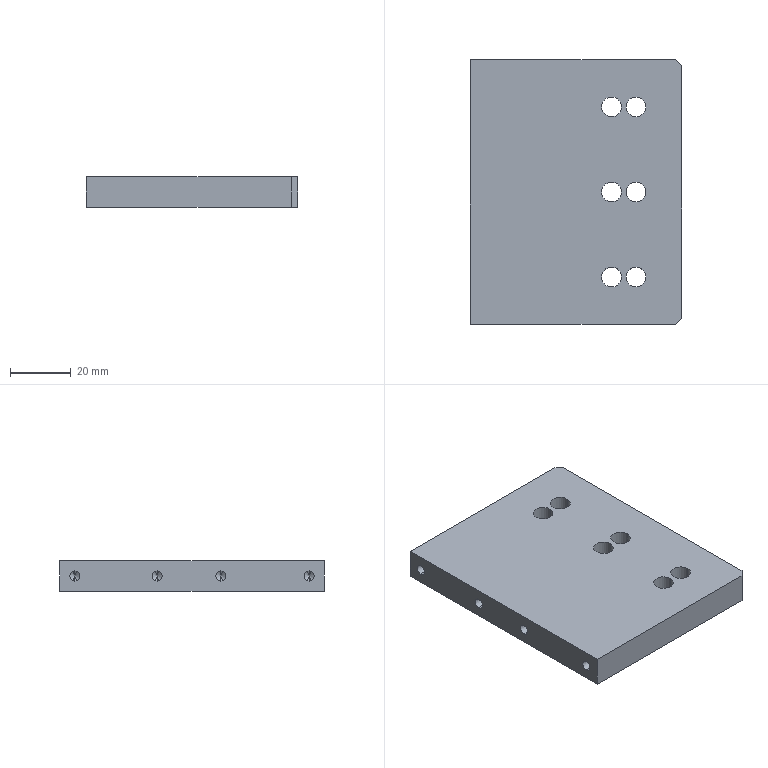Part | STEP file | 02-09 moving fixing plate | 1 solid | 36 faces | box 69.4 x 87 x 10 mm | volume 57942 mm3 | cylinder 20 | cone 8 | plane 8 | commonest cylinder face diameters 6.5 x12 3.3 x8
STEP:
#1=CARTESIAN_POINT('',(14.95,-28.,10.));
#2=VERTEX_POINT('',#1);
#3=CARTESIAN_POINT('',(8.45,-28.,10.));
#4=VERTEX_POINT('',#3);
#5=CARTESIAN_POINT('',(11.7,-28.,10.));
#6=DIRECTION('',(0.,0.,-1.));
#7=DIRECTION('',(-1.,0.,0.));
#8=AXIS2_PLACEMENT_3D('',#5,#6,#7);
#9=CIRCLE('',#8,3.25);
#10=EDGE_CURVE('',#2,#4,#9,.T.);
#11=ORIENTED_EDGE('',*,*,#10,.F.);
#12=CARTESIAN_POINT('',(14.95,-28.,0.));
#13=VERTEX_POINT('',#12);
#14=CARTESIAN_POINT('',(14.95,-28.,10.));
#15=DIRECTION('',(0.,0.,-1.));
#16=VECTOR('',#15,1000.);
#17=LINE('',#14,#16);
#18=EDGE_CURVE('',#2,#13,#17,.T.);
#19=ORIENTED_EDGE('',*,*,#18,.T.);
#20=CARTESIAN_POINT('',(8.45,-28.,0.));
#21=VERTEX_POINT('',#20);
#22=CARTESIAN_POINT('',(11.7,-28.,0.));
#23=DIRECTION('',(0.,0.,-1.));
#24=DIRECTION('',(-1.,0.,0.));
#25=AXIS2_PLACEMENT_3D('',#22,#23,#24);
#26=CIRCLE('',#25,3.25);
#27=EDGE_CURVE('',#13,#21,#26,.T.);
#28=ORIENTED_EDGE('',*,*,#27,.T.);
#29=CARTESIAN_POINT('',(8.45,-28.,10.));
#30=DIRECTION('',(0.,0.,-1.));
#31=VECTOR('',#30,1000.);
#32=LINE('',#29,#31);
#33=EDGE_CURVE('',#4,#21,#32,.T.);
#34=ORIENTED_EDGE('',*,*,#33,.F.);
#35=EDGE_LOOP('',(#11,#19,#28,#34));
#36=FACE_OUTER_BOUND('',#35,.T.);
#37=CARTESIAN_POINT('',(11.7,-28.,10.));
#38=DIRECTION('',(0.,0.,-1.));
#39=DIRECTION('',(-1.,0.,0.));
#40=AXIS2_PLACEMENT_3D('',#37,#38,#39);
#41=CYLINDRICAL_SURFACE('',#40,3.25);
#42=ADVANCED_FACE('',(#36),#41,.F.);
#43=CARTESIAN_POINT('',(14.95,0.,10.));
#44=VERTEX_POINT('',#43);
#45=CARTESIAN_POINT('',(8.45,0.,10.));
#46=VERTEX_POINT('',#45);
#47=CARTESIAN_POINT('',(11.7,0.,10.));
#48=DIRECTION('',(0.,0.,-1.));
#49=DIRECTION('',(-1.,0.,0.));
#50=AXIS2_PLACEMENT_3D('',#47,#48,#49);
#51=CIRCLE('',#50,3.25);
#52=EDGE_CURVE('',#44,#46,#51,.T.);
#53=ORIENTED_EDGE('',*,*,#52,.F.);
#54=CARTESIAN_POINT('',(14.95,0.,0.));
#55=VERTEX_POINT('',#54);
#56=CARTESIAN_POINT('',(14.95,0.,10.));
#57=DIRECTION('',(0.,0.,-1.));
#58=VECTOR('',#57,1000.);
#59=LINE('',#56,#58);
#60=EDGE_CURVE('',#44,#55,#59,.T.);
#61=ORIENTED_EDGE('',*,*,#60,.T.);
#62=CARTESIAN_POINT('',(8.45,0.,0.));
#63=VERTEX_POINT('',#62);
#64=CARTESIAN_POINT('',(11.7,0.,0.));
#65=DIRECTION('',(0.,0.,-1.));
#66=DIRECTION('',(-1.,0.,0.));
#67=AXIS2_PLACEMENT_3D('',#64,#65,#66);
#68=CIRCLE('',#67,3.25);
#69=EDGE_CURVE('',#55,#63,#68,.T.);
#70=ORIENTED_EDGE('',*,*,#69,.T.);
#71=CARTESIAN_POINT('',(8.45,0.,10.));
#72=DIRECTION('',(0.,0.,-1.));
#73=VECTOR('',#72,1000.);
#74=LINE('',#71,#73);
#75=EDGE_CURVE('',#46,#63,#74,.T.);
#76=ORIENTED_EDGE('',*,*,#75,.F.);
#77=EDGE_LOOP('',(#53,#61,#70,#76));
#78=FACE_OUTER_BOUND('',#77,.T.);
#79=CARTESIAN_POINT('',(11.7,0.,10.));
#80=DIRECTION('',(0.,0.,-1.));
#81=DIRECTION('',(-1.,0.,0.));
#82=AXIS2_PLACEMENT_3D('',#79,#80,#81);
#83=CYLINDRICAL_SURFACE('',#82,3.25);
#84=ADVANCED_FACE('',(#78),#83,.F.);
#85=CARTESIAN_POINT('',(14.95,28.,10.));
#86=VERTEX_POINT('',#85);
#87=CARTESIAN_POINT('',(8.45,28.,10.));
#88=VERTEX_POINT('',#87);
#89=CARTESIAN_POINT('',(11.7,28.,10.));
#90=DIRECTION('',(0.,0.,-1.));
#91=DIRECTION('',(-1.,0.,0.));
#92=AXIS2_PLACEMENT_3D('',#89,#90,#91);
#93=CIRCLE('',#92,3.25);
#94=EDGE_CURVE('',#86,#88,#93,.T.);
#95=ORIENTED_EDGE('',*,*,#94,.F.);
#96=CARTESIAN_POINT('',(14.95,28.,0.));
#97=VERTEX_POINT('',#96);
#98=CARTESIAN_POINT('',(14.95,28.,10.));
#99=DIRECTION('',(0.,0.,-1.));
#100=VECTOR('',#99,1000.);
#101=LINE('',#98,#100);
#102=EDGE_CURVE('',#86,#97,#101,.T.);
#103=ORIENTED_EDGE('',*,*,#102,.T.);
#104=CARTESIAN_POINT('',(8.45,28.,0.));
#105=VERTEX_POINT('',#104);
#106=CARTESIAN_POINT('',(11.7,28.,0.));
#107=DIRECTION('',(0.,0.,-1.));
#108=DIRECTION('',(-1.,0.,0.));
#109=AXIS2_PLACEMENT_3D('',#106,#107,#108);
#110=CIRCLE('',#109,3.25);
#111=EDGE_CURVE('',#97,#105,#110,.T.);
#112=ORIENTED_EDGE('',*,*,#111,.T.);
#113=CARTESIAN_POINT('',(8.45,28.,10.));
#114=DIRECTION('',(0.,0.,-1.));
#115=VECTOR('',#114,1000.);
#116=LINE('',#113,#115);
#117=EDGE_CURVE('',#88,#105,#116,.T.);
#118=ORIENTED_EDGE('',*,*,#117,.F.);
#119=EDGE_LOOP('',(#95,#103,#112,#118));
#120=FACE_OUTER_BOUND('',#119,.T.);
#121=CARTESIAN_POINT('',(11.7,28.,10.));
#122=DIRECTION('',(0.,0.,-1.));
#123=DIRECTION('',(-1.,0.,0.));
#124=AXIS2_PLACEMENT_3D('',#121,#122,#123);
#125=CYLINDRICAL_SURFACE('',#124,3.25);
#126=ADVANCED_FACE('',(#120),#125,.F.);
#127=CARTESIAN_POINT('',(16.45,-28.,0.));
#128=VERTEX_POINT('',#127);
#129=CARTESIAN_POINT('',(22.95,-28.,0.));
#130=VERTEX_POINT('',#129);
#131=CARTESIAN_POINT('',(19.7,-28.,0.));
#132=DIRECTION('',(0.,0.,1.));
#133=DIRECTION('',(1.,0.,0.));
#134=AXIS2_PLACEMENT_3D('',#131,#132,#133);
#135=CIRCLE('',#134,3.25);
#136=EDGE_CURVE('',#128,#130,#135,.T.);
#137=ORIENTED_EDGE('',*,*,#136,.F.);
#138=CARTESIAN_POINT('',(16.45,-28.,10.));
#139=VERTEX_POINT('',#138);
#140=CARTESIAN_POINT('',(16.45,-28.,0.));
#141=DIRECTION('',(0.,0.,1.));
#142=VECTOR('',#141,1000.);
#143=LINE('',#140,#142);
#144=EDGE_CURVE('',#128,#139,#143,.T.);
#145=ORIENTED_EDGE('',*,*,#144,.T.);
#146=CARTESIAN_POINT('',(22.95,-28.,10.));
#147=VERTEX_POINT('',#146);
#148=CARTESIAN_POINT('',(19.7,-28.,10.));
#149=DIRECTION('',(0.,0.,1.));
#150=DIRECTION('',(1.,0.,0.));
#151=AXIS2_PLACEMENT_3D('',#148,#149,#150);
#152=CIRCLE('',#151,3.25);
#153=EDGE_CURVE('',#139,#147,#152,.T.);
#154=ORIENTED_EDGE('',*,*,#153,.T.);
#155=CARTESIAN_POINT('',(22.95,-28.,0.));
#156=DIRECTION('',(0.,0.,1.));
#157=VECTOR('',#156,1000.);
#158=LINE('',#155,#157);
#159=EDGE_CURVE('',#130,#147,#158,.T.);
#160=ORIENTED_EDGE('',*,*,#159,.F.);
#161=EDGE_LOOP('',(#137,#145,#154,#160));
#162=FACE_OUTER_BOUND('',#161,.T.);
#163=CARTESIAN_POINT('',(19.7,-28.,0.));
#164=DIRECTION('',(0.,0.,1.));
#165=DIRECTION('',(1.,0.,0.));
#166=AXIS2_PLACEMENT_3D('',#163,#164,#165);
#167=CYLINDRICAL_SURFACE('',#166,3.25);
#168=ADVANCED_FACE('',(#162),#167,.F.);
#169=CARTESIAN_POINT('',(16.45,0.,0.));
#170=VERTEX_POINT('',#169);
#171=CARTESIAN_POINT('',(22.95,0.,0.));
#172=VERTEX_POINT('',#171);
#173=CARTESIAN_POINT('',(19.7,0.,0.));
#174=DIRECTION('',(0.,0.,1.));
#175=DIRECTION('',(1.,0.,0.));
#176=AXIS2_PLACEMENT_3D('',#173,#174,#175);
#177=CIRCLE('',#176,3.25);
#178=EDGE_CURVE('',#170,#172,#177,.T.);
#179=ORIENTED_EDGE('',*,*,#178,.F.);
#180=CARTESIAN_POINT('',(16.45,0.,10.));
#181=VERTEX_POINT('',#180);
#182=CARTESIAN_POINT('',(16.45,0.,0.));
#183=DIRECTION('',(0.,0.,1.));
#184=VECTOR('',#183,1000.);
#185=LINE('',#182,#184);
#186=EDGE_CURVE('',#170,#181,#185,.T.);
#187=ORIENTED_EDGE('',*,*,#186,.T.);
#188=CARTESIAN_POINT('',(22.95,0.,10.));
#189=VERTEX_POINT('',#188);
#190=CARTESIAN_POINT('',(19.7,0.,10.));
#191=DIRECTION('',(0.,0.,1.));
#192=DIRECTION('',(1.,0.,0.));
#193=AXIS2_PLACEMENT_3D('',#190,#191,#192);
#194=CIRCLE('',#193,3.25);
#195=EDGE_CURVE('',#181,#189,#194,.T.);
#196=ORIENTED_EDGE('',*,*,#195,.T.);
#197=CARTESIAN_POINT('',(22.95,0.,0.));
#198=DIRECTION('',(0.,0.,1.));
#199=VECTOR('',#198,1000.);
#200=LINE('',#197,#199);
#201=EDGE_CURVE('',#172,#189,#200,.T.);
#202=ORIENTED_EDGE('',*,*,#201,.F.);
#203=EDGE_LOOP('',(#179,#187,#196,#202));
#204=FACE_OUTER_BOUND('',#203,.T.);
#205=CARTESIAN_POINT('',(19.7,0.,0.));
#206=DIRECTION('',(0.,0.,1.));
#207=DIRECTION('',(1.,0.,0.));
#208=AXIS2_PLACEMENT_3D('',#205,#206,#207);
#209=CYLINDRICAL_SURFACE('',#208,3.25);
#210=ADVANCED_FACE('',(#204),#209,.F.);
#211=CARTESIAN_POINT('',(16.45,28.,0.));
#212=VERTEX_POINT('',#211);
#213=CARTESIAN_POINT('',(22.95,28.,0.));
#214=VERTEX_POINT('',#213);
#215=CARTESIAN_POINT('',(19.7,28.,0.));
#216=DIRECTION('',(0.,0.,1.));
#217=DIRECTION('',(1.,0.,0.));
#218=AXIS2_PLACEMENT_3D('',#215,#216,#217);
#219=CIRCLE('',#218,3.25);
#220=EDGE_CURVE('',#212,#214,#219,.T.);
#221=ORIENTED_EDGE('',*,*,#220,.F.);
#222=CARTESIAN_POINT('',(16.45,28.,10.));
#223=VERTEX_POINT('',#222);
#224=CARTESIAN_POINT('',(16.45,28.,0.));
#225=DIRECTION('',(0.,0.,1.));
#226=VECTOR('',#225,1000.);
#227=LINE('',#224,#226);
#228=EDGE_CURVE('',#212,#223,#227,.T.);
#229=ORIENTED_EDGE('',*,*,#228,.T.);
#230=CARTESIAN_POINT('',(22.95,28.,10.));
#231=VERTEX_POINT('',#230);
#232=CARTESIAN_POINT('',(19.7,28.,10.));
#233=DIRECTION('',(0.,0.,1.));
#234=DIRECTION('',(1.,0.,0.));
#235=AXIS2_PLACEMENT_3D('',#232,#233,#234);
#236=CIRCLE('',#235,3.25);
#237=EDGE_CURVE('',#223,#231,#236,.T.);
#238=ORIENTED_EDGE('',*,*,#237,.T.);
#239=CARTESIAN_POINT('',(22.95,28.,0.));
#240=DIRECTION('',(0.,0.,1.));
#241=VECTOR('',#240,1000.);
#242=LINE('',#239,#241);
#243=EDGE_CURVE('',#214,#231,#242,.T.);
#244=ORIENTED_EDGE('',*,*,#243,.F.);
#245=EDGE_LOOP('',(#221,#229,#238,#244));
#246=FACE_OUTER_BOUND('',#245,.T.);
#247=CARTESIAN_POINT('',(19.7,28.,0.));
#248=DIRECTION('',(0.,0.,1.));
#249=DIRECTION('',(1.,0.,0.));
#250=AXIS2_PLACEMENT_3D('',#247,#248,#249);
#251=CYLINDRICAL_SURFACE('',#250,3.25);
#252=ADVANCED_FACE('',(#246),#251,.F.);
#253=CARTESIAN_POINT('',(-23.2,38.5,3.35));
#254=VERTEX_POINT('',#253);
#255=CARTESIAN_POINT('',(-23.2,38.5,6.65));
#256=VERTEX_POINT('',#255);
#257=CARTESIAN_POINT('',(-23.2,38.5,5.));
#258=DIRECTION('',(-1.,0.,0.));
#259=DIRECTION('',(0.,0.,1.));
#260=AXIS2_PLACEMENT_3D('',#257,#258,#259);
#261=CIRCLE('',#260,1.65);
#262=EDGE_CURVE('',#254,#256,#261,.T.);
#263=ORIENTED_EDGE('',*,*,#262,.F.);
#264=CARTESIAN_POINT('',(-34.7,38.5,3.35));
#265=VERTEX_POINT('',#264);
#266=CARTESIAN_POINT('',(-34.7,38.5,3.35));
#267=DIRECTION('',(-1.,0.,0.));
#268=VECTOR('',#267,1000.);
#269=LINE('',#266,#268);
#270=EDGE_CURVE('',#254,#265,#269,.T.);
#271=ORIENTED_EDGE('',*,*,#270,.T.);
#272=CARTESIAN_POINT('',(-34.7,38.5,6.65));
#273=VERTEX_POINT('',#272);
#274=CARTESIAN_POINT('',(-34.7,38.5,5.));
#275=DIRECTION('',(-1.,0.,0.));
#276=DIRECTION('',(0.,0.,1.));
#277=AXIS2_PLACEMENT_3D('',#274,#275,#276);
#278=CIRCLE('',#277,1.65);
#279=EDGE_CURVE('',#265,#273,#278,.T.);
#280=ORIENTED_EDGE('',*,*,#279,.T.);
#281=CARTESIAN_POINT('',(-34.7,38.5,6.65));
#282=DIRECTION('',(-1.,0.,0.));
#283=VECTOR('',#282,1000.);
#284=LINE('',#281,#283);
#285=EDGE_CURVE('',#256,#273,#284,.T.);
#286=ORIENTED_EDGE('',*,*,#285,.F.);
#287=EDGE_LOOP('',(#263,#271,#280,#286));
#288=FACE_OUTER_BOUND('',#287,.T.);
#289=CARTESIAN_POINT('',(-34.7,38.5,5.));
#290=DIRECTION('',(-1.,0.,0.));
#291=DIRECTION('',(0.,0.,1.));
#292=AXIS2_PLACEMENT_3D('',#289,#290,#291);
#293=CYLINDRICAL_SURFACE('',#292,1.65);
#294=ADVANCED_FACE('',(#288),#293,.F.);
#295=CARTESIAN_POINT('',(-22.209,38.5,5.));
#296=VERTEX_POINT('',#295);
#297=CARTESIAN_POINT('',(-23.2,38.5,6.65));
#298=DIRECTION('',(-0.515,0.,0.8572));
#299=VECTOR('',#298,1000.);
#300=LINE('',#297,#299);
#301=EDGE_CURVE('',#296,#256,#300,.T.);
#302=ORIENTED_EDGE('',*,*,#301,.F.);
#303=CARTESIAN_POINT('',(-23.2,38.5,3.35));
#304=DIRECTION('',(-0.515,0.,-0.8572));
#305=VECTOR('',#304,1000.);
#306=LINE('',#303,#305);
#307=EDGE_CURVE('',#296,#254,#306,.T.);
#308=ORIENTED_EDGE('',*,*,#307,.T.);
#309=ORIENTED_EDGE('',*,*,#262,.T.);
#310=EDGE_LOOP('',(#302,#308,#309));
#311=FACE_OUTER_BOUND('',#310,.T.);
#312=CARTESIAN_POINT('',(-23.2,38.5,5.));
#313=DIRECTION('',(-1.,0.,0.));
#314=DIRECTION('',(0.,0.,1.));
#315=AXIS2_PLACEMENT_3D('',#312,#313,#314);
#316=CONICAL_SURFACE('',#315,1.65,1.03);
#317=ADVANCED_FACE('',(#311),#316,.F.);
#318=CARTESIAN_POINT('',(-23.2,-38.5,3.35));
#319=VERTEX_POINT('',#318);
#320=CARTESIAN_POINT('',(-23.2,-38.5,6.65));
#321=VERTEX_POINT('',#320);
#322=CARTESIAN_POINT('',(-23.2,-38.5,5.));
#323=DIRECTION('',(-1.,0.,0.));
#324=DIRECTION('',(0.,0.,1.));
#325=AXIS2_PLACEMENT_3D('',#322,#323,#324);
#326=CIRCLE('',#325,1.65);
#327=EDGE_CURVE('',#319,#321,#326,.T.);
#328=ORIENTED_EDGE('',*,*,#327,.F.);
#329=CARTESIAN_POINT('',(-34.7,-38.5,3.35));
#330=VERTEX_POINT('',#329);
#331=CARTESIAN_POINT('',(-34.7,-38.5,3.35));
#332=DIRECTION('',(-1.,0.,0.));
#333=VECTOR('',#332,1000.);
#334=LINE('',#331,#333);
#335=EDGE_CURVE('',#319,#330,#334,.T.);
#336=ORIENTED_EDGE('',*,*,#335,.T.);
#337=CARTESIAN_POINT('',(-34.7,-38.5,6.65));
#338=VERTEX_POINT('',#337);
#339=CARTESIAN_POINT('',(-34.7,-38.5,5.));
#340=DIRECTION('',(-1.,0.,0.));
#341=DIRECTION('',(0.,0.,1.));
#342=AXIS2_PLACEMENT_3D('',#339,#340,#341);
#343=CIRCLE('',#342,1.65);
#344=EDGE_CURVE('',#330,#338,#343,.T.);
#345=ORIENTED_EDGE('',*,*,#344,.T.);
#346=CARTESIAN_POINT('',(-34.7,-38.5,6.65));
#347=DIRECTION('',(-1.,0.,0.));
#348=VECTOR('',#347,1000.);
#349=LINE('',#346,#348);
#350=EDGE_CURVE('',#321,#338,#349,.T.);
#351=ORIENTED_EDGE('',*,*,#350,.F.);
#352=EDGE_LOOP('',(#328,#336,#345,#351));
#353=FACE_OUTER_BOUND('',#352,.T.);
#354=CARTESIAN_POINT('',(-34.7,-38.5,5.));
#355=DIRECTION('',(-1.,0.,0.));
#356=DIRECTION('',(0.,0.,1.));
#357=AXIS2_PLACEMENT_3D('',#354,#355,#356);
#358=CYLINDRICAL_SURFACE('',#357,1.65);
#359=ADVANCED_FACE('',(#353),#358,.F.);
#360=CARTESIAN_POINT('',(-22.209,-38.5,5.));
#361=VERTEX_POINT('',#360);
#362=CARTESIAN_POINT('',(-23.2,-38.5,6.65));
#363=DIRECTION('',(-0.515,0.,0.8572));
#364=VECTOR('',#363,1000.);
#365=LINE('',#362,#364);
#366=EDGE_CURVE('',#361,#321,#365,.T.);
#367=ORIENTED_EDGE('',*,*,#366,.F.);
#368=CARTESIAN_POINT('',(-23.2,-38.5,3.35));
#369=DIRECTION('',(-0.515,0.,-0.8572));
#370=VECTOR('',#369,1000.);
#371=LINE('',#368,#370);
#372=EDGE_CURVE('',#361,#319,#371,.T.);
#373=ORIENTED_EDGE('',*,*,#372,.T.);
#374=ORIENTED_EDGE('',*,*,#327,.T.);
#375=EDGE_LOOP('',(#367,#373,#374));
#376=FACE_OUTER_BOUND('',#375,.T.);
#377=CARTESIAN_POINT('',(-23.2,-38.5,5.));
#378=DIRECTION('',(-1.,0.,0.));
#379=DIRECTION('',(0.,0.,1.));
#380=AXIS2_PLACEMENT_3D('',#377,#378,#379);
#381=CONICAL_SURFACE('',#380,1.65,1.03);
#382=ADVANCED_FACE('',(#376),#381,.F.);
#383=CARTESIAN_POINT('',(-23.2,11.5,3.35));
#384=VERTEX_POINT('',#383);
#385=CARTESIAN_POINT('',(-23.2,11.5,6.65));
#386=VERTEX_POINT('',#385);
#387=CARTESIAN_POINT('',(-23.2,11.5,5.));
#388=DIRECTION('',(-1.,0.,0.));
#389=DIRECTION('',(0.,0.,1.));
#390=AXIS2_PLACEMENT_3D('',#387,#388,#389);
#391=CIRCLE('',#390,1.65);
#392=EDGE_CURVE('',#384,#386,#391,.T.);
#393=ORIENTED_EDGE('',*,*,#392,.F.);
#394=CARTESIAN_POINT('',(-34.7,11.5,3.35));
#395=VERTEX_POINT('',#394);
#396=CARTESIAN_POINT('',(-34.7,11.5,3.35));
#397=DIRECTION('',(-1.,0.,0.));
#398=VECTOR('',#397,1000.);
#399=LINE('',#396,#398);
#400=EDGE_CURVE('',#384,#395,#399,.T.);
#401=ORIENTED_EDGE('',*,*,#400,.T.);
#402=CARTESIAN_POINT('',(-34.7,11.5,6.65));
#403=VERTEX_POINT('',#402);
#404=CARTESIAN_POINT('',(-34.7,11.5,5.));
#405=DIRECTION('',(-1.,0.,0.));
#406=DIRECTION('',(0.,0.,1.));
#407=AXIS2_PLACEMENT_3D('',#404,#405,#406);
#408=CIRCLE('',#407,1.65);
#409=EDGE_CURVE('',#395,#403,#408,.T.);
#410=ORIENTED_EDGE('',*,*,#409,.T.);
#411=CARTESIAN_POINT('',(-34.7,11.5,6.65));
#412=DIRECTION('',(-1.,0.,0.));
#413=VECTOR('',#412,1000.);
#414=LINE('',#411,#413);
#415=EDGE_CURVE('',#386,#403,#414,.T.);
#416=ORIENTED_EDGE('',*,*,#415,.F.);
#417=EDGE_LOOP('',(#393,#401,#410,#416));
#418=FACE_OUTER_BOUND('',#417,.T.);
#419=CARTESIAN_POINT('',(-34.7,11.5,5.));
#420=DIRECTION('',(-1.,0.,0.));
#421=DIRECTION('',(0.,0.,1.));
#422=AXIS2_PLACEMENT_3D('',#419,#420,#421);
#423=CYLINDRICAL_SURFACE('',#422,1.65);
#424=ADVANCED_FACE('',(#418),#423,.F.);
#425=CARTESIAN_POINT('',(-22.209,11.5,5.));
#426=VERTEX_POINT('',#425);
#427=CARTESIAN_POINT('',(-23.2,11.5,6.65));
#428=DIRECTION('',(-0.515,0.,0.8572));
#429=VECTOR('',#428,1000.);
#430=LINE('',#427,#429);
#431=EDGE_CURVE('',#426,#386,#430,.T.);
#432=ORIENTED_EDGE('',*,*,#431,.F.);
#433=CARTESIAN_POINT('',(-23.2,11.5,3.35));
#434=DIRECTION('',(-0.515,0.,-0.8572));
#435=VECTOR('',#434,1000.);
#436=LINE('',#433,#435);
#437=EDGE_CURVE('',#426,#384,#436,.T.);
#438=ORIENTED_EDGE('',*,*,#437,.T.);
#439=ORIENTED_EDGE('',*,*,#392,.T.);
#440=EDGE_LOOP('',(#432,#438,#439));
#441=FACE_OUTER_BOUND('',#440,.T.);
#442=CARTESIAN_POINT('',(-23.2,11.5,5.));
#443=DIRECTION('',(-1.,0.,0.));
#444=DIRECTION('',(0.,0.,1.));
#445=AXIS2_PLACEMENT_3D('',#442,#443,#444);
#446=CONICAL_SURFACE('',#445,1.65,1.03);
#447=ADVANCED_FACE('',(#441),#446,.F.);
#448=CARTESIAN_POINT('',(-23.2,-9.5,3.35));
#449=VERTEX_POINT('',#448);
#450=CARTESIAN_POINT('',(-23.2,-9.5,6.65));
#451=VERTEX_POINT('',#450);
#452=CARTESIAN_POINT('',(-23.2,-9.5,5.));
#453=DIRECTION('',(-1.,0.,0.));
#454=DIRECTION('',(0.,0.,1.));
#455=AXIS2_PLACEMENT_3D('',#452,#453,#454);
#456=CIRCLE('',#455,1.65);
#457=EDGE_CURVE('',#449,#451,#456,.T.);
#458=ORIENTED_EDGE('',*,*,#457,.F.);
#459=CARTESIAN_POINT('',(-34.7,-9.5,3.35));
#460=VERTEX_POINT('',#459);
#461=CARTESIAN_POINT('',(-34.7,-9.5,3.35));
#462=DIRECTION('',(-1.,0.,0.));
#463=VECTOR('',#462,1000.);
#464=LINE('',#461,#463);
#465=EDGE_CURVE('',#449,#460,#464,.T.);
#466=ORIENTED_EDGE('',*,*,#465,.T.);
#467=CARTESIAN_POINT('',(-34.7,-9.5,6.65));
#468=VERTEX_POINT('',#467);
#469=CARTESIAN_POINT('',(-34.7,-9.5,5.));
#470=DIRECTION('',(-1.,0.,0.));
#471=DIRECTION('',(0.,0.,1.));
#472=AXIS2_PLACEMENT_3D('',#469,#470,#471);
#473=CIRCLE('',#472,1.65);
#474=EDGE_CURVE('',#460,#468,#473,.T.);
#475=ORIENTED_EDGE('',*,*,#474,.T.);
#476=CARTESIAN_POINT('',(-34.7,-9.5,6.65));
#477=DIRECTION('',(-1.,0.,0.));
#478=VECTOR('',#477,1000.);
#479=LINE('',#476,#478);
#480=EDGE_CURVE('',#451,#468,#479,.T.);
#481=ORIENTED_EDGE('',*,*,#480,.F.);
#482=EDGE_LOOP('',(#458,#466,#475,#481));
#483=FACE_OUTER_BOUND('',#482,.T.);
#484=CARTESIAN_POINT('',(-34.7,-9.5,5.));
#485=DIRECTION('',(-1.,0.,0.));
#486=DIRECTION('',(0.,0.,1.));
#487=AXIS2_PLACEMENT_3D('',#484,#485,#486);
#488=CYLINDRICAL_SURFACE('',#487,1.65);
#489=ADVANCED_FACE('',(#483),#488,.F.);
#490=CARTESIAN_POINT('',(-22.209,-9.5,5.));
#491=VERTEX_POINT('',#490);
#492=CARTESIAN_POINT('',(-23.2,-9.5,6.65));
#493=DIRECTION('',(-0.515,0.,0.8572));
#494=VECTOR('',#493,1000.);
#495=LINE('',#492,#494);
#496=EDGE_CURVE('',#491,#451,#495,.T.);
#497=ORIENTED_EDGE('',*,*,#496,.F.);
#498=CARTESIAN_POINT('',(-23.2,-9.5,3.35));
#499=DIRECTION('',(-0.515,0.,-0.8572));
#500=VECTOR('',#499,1000.);
#501=LINE('',#498,#500);
#502=EDGE_CURVE('',#491,#449,#501,.T.);
#503=ORIENTED_EDGE('',*,*,#502,.T.);
#504=ORIENTED_EDGE('',*,*,#457,.T.);
#505=EDGE_LOOP('',(#497,#503,#504));
#506=FACE_OUTER_BOUND('',#505,.T.);
#507=CARTESIAN_POINT('',(-23.2,-9.5,5.));
#508=DIRECTION('',(-1.,0.,0.));
#509=DIRECTION('',(0.,0.,1.));
#510=AXIS2_PLACEMENT_3D('',#507,#508,#509);
#511=CONICAL_SURFACE('',#510,1.65,1.03);
#512=ADVANCED_FACE('',(#506),#511,.F.);
#513=CARTESIAN_POINT('',(34.7,-41.5,0.));
#514=VERTEX_POINT('',#513);
#515=CARTESIAN_POINT('',(34.7,41.5,0.));
#516=VERTEX_POINT('',#515);
#517=CARTESIAN_POINT('',(34.7,43.5,0.));
#518=DIRECTION('',(0.,1.,0.));
#519=VECTOR('',#518,1000.);
#520=LINE('',#517,#519);
#521=EDGE_CURVE('',#514,#516,#520,.T.);
#522=ORIENTED_EDGE('',*,*,#521,.T.);
#523=CARTESIAN_POINT('',(34.7,41.5,10.));
#524=VERTEX_POINT('',#523);
#525=CARTESIAN_POINT('',(34.7,41.5,10.));
#526=DIRECTION('',(0.,0.,1.));
#527=VECTOR('',#526,1000.);
#528=LINE('',#525,#527);
#529=EDGE_CURVE('',#516,#524,#528,.T.);
#530=ORIENTED_EDGE('',*,*,#529,.T.);
#531=CARTESIAN_POINT('',(34.7,-41.5,10.));
#532=VERTEX_POINT('',#531);
#533=CARTESIAN_POINT('',(34.7,43.5,10.));
#534=DIRECTION('',(0.,1.,0.));
#535=VECTOR('',#534,1000.);
#536=LINE('',#533,#535);
#537=EDGE_CURVE('',#532,#524,#536,.T.);
#538=ORIENTED_EDGE('',*,*,#537,.F.);
#539=CARTESIAN_POINT('',(34.7,-41.5,10.));
#540=DIRECTION('',(0.,0.,-1.));
#541=VECTOR('',#540,1000.);
#542=LINE('',#539,#541);
#543=EDGE_CURVE('',#532,#514,#542,.T.);
#544=ORIENTED_EDGE('',*,*,#543,.T.);
#545=EDGE_LOOP('',(#522,#530,#538,#544));
#546=FACE_OUTER_BOUND('',#545,.T.);
#547=CARTESIAN_POINT('',(34.7,43.5,10.));
#548=DIRECTION('',(-1.,0.,0.));
#549=DIRECTION('',(0.,-1.,0.));
#550=AXIS2_PLACEMENT_3D('',#547,#548,#549);
#551=PLANE('',#550);
#552=ADVANCED_FACE('',(#546),#551,.F.);
#553=CARTESIAN_POINT('',(32.7,43.5,10.));
#554=VERTEX_POINT('',#553);
#555=CARTESIAN_POINT('',(-34.7,43.5,10.));
#556=VERTEX_POINT('',#555);
#557=CARTESIAN_POINT('',(-34.7,43.5,10.));
#558=DIRECTION('',(-1.,0.,0.));
#559=VECTOR('',#558,1000.);
#560=LINE('',#557,#559);
#561=EDGE_CURVE('',#554,#556,#560,.T.);
#562=ORIENTED_EDGE('',*,*,#561,.F.);
#563=CARTESIAN_POINT('',(32.7,43.5,0.));
#564=VERTEX_POINT('',#563);
#565=CARTESIAN_POINT('',(32.7,43.5,10.));
#566=DIRECTION('',(0.,0.,-1.));
#567=VECTOR('',#566,1000.);
#568=LINE('',#565,#567);
#569=EDGE_CURVE('',#554,#564,#568,.T.);
#570=ORIENTED_EDGE('',*,*,#569,.T.);
#571=CARTESIAN_POINT('',(-34.7,43.5,0.));
#572=VERTEX_POINT('',#571);
#573=CARTESIAN_POINT('',(-34.7,43.5,0.));
#574=DIRECTION('',(-1.,0.,0.));
#575=VECTOR('',#574,1000.);
#576=LINE('',#573,#575);
#577=EDGE_CURVE('',#564,#572,#576,.T.);
#578=ORIENTED_EDGE('',*,*,#577,.T.);
#579=CARTESIAN_POINT('',(-34.7,43.5,10.));
#580=DIRECTION('',(0.,0.,-1.));
#581=VECTOR('',#580,1000.);
#582=LINE('',#579,#581);
#583=EDGE_CURVE('',#556,#572,#582,.T.);
#584=ORIENTED_EDGE('',*,*,#583,.F.);
#585=EDGE_LOOP('',(#562,#570,#578,#584));
#586=FACE_OUTER_BOUND('',#585,.T.);
#587=CARTESIAN_POINT('',(-34.7,43.5,10.));
#588=DIRECTION('',(0.,-1.,0.));
#589=DIRECTION('',(0.,0.,-1.));
#590=AXIS2_PLACEMENT_3D('',#587,#588,#589);
#591=PLANE('',#590);
#592=ADVANCED_FACE('',(#586),#591,.F.);
#593=CARTESIAN_POINT('',(-34.7,38.5,5.));
#594=DIRECTION('',(-1.,0.,0.));
#595=DIRECTION('',(0.,0.,1.));
#596=AXIS2_PLACEMENT_3D('',#593,#594,#595);
#597=CIRCLE('',#596,1.65);
#598=EDGE_CURVE('',#273,#265,#597,.T.);
#599=ORIENTED_EDGE('',*,*,#598,.F.);
#600=ORIENTED_EDGE('',*,*,#279,.F.);
#601=EDGE_LOOP('',(#599,#600));
#602=FACE_BOUND('',#601,.T.);
#603=CARTESIAN_POINT('',(-34.7,-38.5,5.));
#604=DIRECTION('',(-1.,0.,0.));
#605=DIRECTION('',(0.,0.,1.));
#606=AXIS2_PLACEMENT_3D('',#603,#604,#605);
#607=CIRCLE('',#606,1.65);
#608=EDGE_CURVE('',#338,#330,#607,.T.);
#609=ORIENTED_EDGE('',*,*,#608,.F.);
#610=ORIENTED_EDGE('',*,*,#344,.F.);
#611=EDGE_LOOP('',(#609,#610));
#612=FACE_BOUND('',#611,.T.);
#613=CARTESIAN_POINT('',(-34.7,11.5,5.));
#614=DIRECTION('',(-1.,0.,0.));
#615=DIRECTION('',(0.,0.,1.));
#616=AXIS2_PLACEMENT_3D('',#613,#614,#615);
#617=CIRCLE('',#616,1.65);
#618=EDGE_CURVE('',#403,#395,#617,.T.);
#619=ORIENTED_EDGE('',*,*,#618,.F.);
#620=ORIENTED_EDGE('',*,*,#409,.F.);
#621=EDGE_LOOP('',(#619,#620));
#622=FACE_BOUND('',#621,.T.);
#623=CARTESIAN_POINT('',(-34.7,-9.5,5.));
#624=DIRECTION('',(-1.,0.,0.));
#625=DIRECTION('',(0.,0.,1.));
#626=AXIS2_PLACEMENT_3D('',#623,#624,#625);
#627=CIRCLE('',#626,1.65);
#628=EDGE_CURVE('',#468,#460,#627,.T.);
#629=ORIENTED_EDGE('',*,*,#628,.F.);
#630=ORIENTED_EDGE('',*,*,#474,.F.);
#631=EDGE_LOOP('',(#629,#630));
#632=FACE_BOUND('',#631,.T.);
#633=CARTESIAN_POINT('',(-34.7,-43.5,0.));
#634=VERTEX_POINT('',#633);
#635=CARTESIAN_POINT('',(-34.7,43.5,0.));
#636=DIRECTION('',(0.,-1.,0.));
#637=VECTOR('',#636,1000.);
#638=LINE('',#635,#637);
#639=EDGE_CURVE('',#572,#634,#638,.T.);
#640=ORIENTED_EDGE('',*,*,#639,.T.);
#641=CARTESIAN_POINT('',(-34.7,-43.5,10.));
#642=VERTEX_POINT('',#641);
#643=CARTESIAN_POINT('',(-34.7,-43.5,10.));
#644=DIRECTION('',(0.,0.,-1.));
#645=VECTOR('',#644,1000.);
#646=LINE('',#643,#645);
#647=EDGE_CURVE('',#642,#634,#646,.T.);
#648=ORIENTED_EDGE('',*,*,#647,.F.);
#649=CARTESIAN_POINT('',(-34.7,43.5,10.));
#650=DIRECTION('',(0.,-1.,0.));
#651=VECTOR('',#650,1000.);
#652=LINE('',#649,#651);
#653=EDGE_CURVE('',#556,#642,#652,.T.);
#654=ORIENTED_EDGE('',*,*,#653,.F.);
#655=ORIENTED_EDGE('',*,*,#583,.T.);
#656=EDGE_LOOP('',(#640,#648,#654,#655));
#657=FACE_OUTER_BOUND('',#656,.T.);
#658=CARTESIAN_POINT('',(-34.7,43.5,10.));
#659=DIRECTION('',(1.,0.,0.));
#660=DIRECTION('',(0.,1.,0.));
#661=AXIS2_PLACEMENT_3D('',#658,#659,#660);
#662=PLANE('',#661);
#663=ADVANCED_FACE('',(#602,#612,#622,#632,#657),#662,.F.);
#664=CARTESIAN_POINT('',(32.7,-43.5,0.));
#665=VERTEX_POINT('',#664);
#666=CARTESIAN_POINT('',(-34.7,-43.5,0.));
#667=DIRECTION('',(1.,0.,0.));
#668=VECTOR('',#667,1000.);
#669=LINE('',#666,#668);
#670=EDGE_CURVE('',#634,#665,#669,.T.);
#671=ORIENTED_EDGE('',*,*,#670,.T.);
#672=CARTESIAN_POINT('',(32.7,-43.5,10.));
#673=VERTEX_POINT('',#672);
#674=CARTESIAN_POINT('',(32.7,-43.5,10.));
#675=DIRECTION('',(0.,0.,1.));
#676=VECTOR('',#675,1000.);
#677=LINE('',#674,#676);
#678=EDGE_CURVE('',#665,#673,#677,.T.);
#679=ORIENTED_EDGE('',*,*,#678,.T.);
#680=CARTESIAN_POINT('',(-34.7,-43.5,10.));
#681=DIRECTION('',(1.,0.,0.));
#682=VECTOR('',#681,1000.);
#683=LINE('',#680,#682);
#684=EDGE_CURVE('',#642,#673,#683,.T.);
#685=ORIENTED_EDGE('',*,*,#684,.F.);
#686=ORIENTED_EDGE('',*,*,#647,.T.);
#687=EDGE_LOOP('',(#671,#679,#685,#686));
#688=FACE_OUTER_BOUND('',#687,.T.);
#689=CARTESIAN_POINT('',(-34.7,-43.5,10.));
#690=DIRECTION('',(0.,1.,0.));
#691=DIRECTION('',(0.,0.,1.));
#692=AXIS2_PLACEMENT_3D('',#689,#690,#691);
#693=PLANE('',#692);
#694=ADVANCED_FACE('',(#688),#693,.F.);
#695=CARTESIAN_POINT('',(11.7,0.,10.));
#696=DIRECTION('',(0.,0.,-1.));
#697=DIRECTION('',(-1.,0.,0.));
#698=AXIS2_PLACEMENT_3D('',#695,#696,#697);
#699=CIRCLE('',#698,3.25);
#700=EDGE_CURVE('',#46,#44,#699,.T.);
#701=ORIENTED_EDGE('',*,*,#700,.T.);
#702=ORIENTED_EDGE('',*,*,#52,.T.);
#703=EDGE_LOOP('',(#701,#702));
#704=FACE_BOUND('',#703,.T.);
#705=CARTESIAN_POINT('',(11.7,28.,10.));
#706=DIRECTION('',(0.,0.,-1.));
#707=DIRECTION('',(-1.,0.,0.));
#708=AXIS2_PLACEMENT_3D('',#705,#706,#707);
#709=CIRCLE('',#708,3.25);
#710=EDGE_CURVE('',#88,#86,#709,.T.);
#711=ORIENTED_EDGE('',*,*,#710,.T.);
#712=ORIENTED_EDGE('',*,*,#94,.T.);
#713=EDGE_LOOP('',(#711,#712));
#714=FACE_BOUND('',#713,.T.);
#715=CARTESIAN_POINT('',(19.7,-28.,10.));
#716=DIRECTION('',(0.,0.,1.));
#717=DIRECTION('',(1.,0.,0.));
#718=AXIS2_PLACEMENT_3D('',#715,#716,#717);
#719=CIRCLE('',#718,3.25);
#720=EDGE_CURVE('',#147,#139,#719,.T.);
#721=ORIENTED_EDGE('',*,*,#720,.F.);
#722=ORIENTED_EDGE('',*,*,#153,.F.);
#723=EDGE_LOOP('',(#721,#722));
#724=FACE_BOUND('',#723,.T.);
#725=CARTESIAN_POINT('',(19.7,0.,10.));
#726=DIRECTION('',(0.,0.,1.));
#727=DIRECTION('',(1.,0.,0.));
#728=AXIS2_PLACEMENT_3D('',#725,#726,#727);
#729=CIRCLE('',#728,3.25);
#730=EDGE_CURVE('',#189,#181,#729,.T.);
#731=ORIENTED_EDGE('',*,*,#730,.F.);
#732=ORIENTED_EDGE('',*,*,#195,.F.);
#733=EDGE_LOOP('',(#731,#732));
#734=FACE_BOUND('',#733,.T.);
#735=CARTESIAN_POINT('',(19.7,28.,10.));
#736=DIRECTION('',(0.,0.,1.));
#737=DIRECTION('',(1.,0.,0.));
#738=AXIS2_PLACEMENT_3D('',#735,#736,#737);
#739=CIRCLE('',#738,3.25);
#740=EDGE_CURVE('',#231,#223,#739,.T.);
#741=ORIENTED_EDGE('',*,*,#740,.F.);
#742=ORIENTED_EDGE('',*,*,#237,.F.);
#743=EDGE_LOOP('',(#741,#742));
#744=FACE_BOUND('',#743,.T.);
#745=ORIENTED_EDGE('',*,*,#537,.T.);
#746=CARTESIAN_POINT('',(77.2,-1.,10.));
#747=DIRECTION('',(-0.7071,0.7071,0.));
#748=VECTOR('',#747,1000.);
#749=LINE('',#746,#748);
#750=EDGE_CURVE('',#524,#554,#749,.T.);
#751=ORIENTED_EDGE('',*,*,#750,.T.);
#752=ORIENTED_EDGE('',*,*,#561,.T.);
#753=ORIENTED_EDGE('',*,*,#653,.T.);
#754=ORIENTED_EDGE('',*,*,#684,.T.);
#755=CARTESIAN_POINT('',(33.7,-42.5,10.));
#756=DIRECTION('',(0.7071,0.7071,0.));
#757=VECTOR('',#756,1000.);
#758=LINE('',#755,#757);
#759=EDGE_CURVE('',#673,#532,#758,.T.);
#760=ORIENTED_EDGE('',*,*,#759,.T.);
#761=EDGE_LOOP('',(#745,#751,#752,#753,#754,#760));
#762=FACE_OUTER_BOUND('',#761,.T.);
#763=CARTESIAN_POINT('',(11.7,-28.,10.));
#764=DIRECTION('',(0.,0.,-1.));
#765=DIRECTION('',(-1.,0.,0.));
#766=AXIS2_PLACEMENT_3D('',#763,#764,#765);
#767=CIRCLE('',#766,3.25);
#768=EDGE_CURVE('',#4,#2,#767,.T.);
#769=ORIENTED_EDGE('',*,*,#768,.T.);
#770=ORIENTED_EDGE('',*,*,#10,.T.);
#771=EDGE_LOOP('',(#769,#770));
#772=FACE_BOUND('',#771,.T.);
#773=CARTESIAN_POINT('',(34.7,-43.5,10.));
#774=DIRECTION('',(0.,0.,1.));
#775=DIRECTION('',(1.,0.,0.));
#776=AXIS2_PLACEMENT_3D('',#773,#774,#775);
#777=PLANE('',#776);
#778=ADVANCED_FACE('',(#704,#714,#724,#734,#744,#762,#772),#777,.T.);
#779=CARTESIAN_POINT('',(11.7,0.,0.));
#780=DIRECTION('',(0.,0.,-1.));
#781=DIRECTION('',(-1.,0.,0.));
#782=AXIS2_PLACEMENT_3D('',#779,#780,#781);
#783=CIRCLE('',#782,3.25);
#784=EDGE_CURVE('',#63,#55,#783,.T.);
#785=ORIENTED_EDGE('',*,*,#784,.F.);
#786=ORIENTED_EDGE('',*,*,#69,.F.);
#787=EDGE_LOOP('',(#785,#786));
#788=FACE_BOUND('',#787,.T.);
#789=CARTESIAN_POINT('',(11.7,28.,0.));
#790=DIRECTION('',(0.,0.,-1.));
#791=DIRECTION('',(-1.,0.,0.));
#792=AXIS2_PLACEMENT_3D('',#789,#790,#791);
#793=CIRCLE('',#792,3.25);
#794=EDGE_CURVE('',#105,#97,#793,.T.);
#795=ORIENTED_EDGE('',*,*,#794,.F.);
#796=ORIENTED_EDGE('',*,*,#111,.F.);
#797=EDGE_LOOP('',(#795,#796));
#798=FACE_BOUND('',#797,.T.);
#799=CARTESIAN_POINT('',(19.7,-28.,0.));
#800=DIRECTION('',(0.,0.,1.));
#801=DIRECTION('',(1.,0.,0.));
#802=AXIS2_PLACEMENT_3D('',#799,#800,#801);
#803=CIRCLE('',#802,3.25);
#804=EDGE_CURVE('',#130,#128,#803,.T.);
#805=ORIENTED_EDGE('',*,*,#804,.T.);
#806=ORIENTED_EDGE('',*,*,#136,.T.);
#807=EDGE_LOOP('',(#805,#806));
#808=FACE_BOUND('',#807,.T.);
#809=CARTESIAN_POINT('',(19.7,0.,0.));
#810=DIRECTION('',(0.,0.,1.));
#811=DIRECTION('',(1.,0.,0.));
#812=AXIS2_PLACEMENT_3D('',#809,#810,#811);
#813=CIRCLE('',#812,3.25);
#814=EDGE_CURVE('',#172,#170,#813,.T.);
#815=ORIENTED_EDGE('',*,*,#814,.T.);
#816=ORIENTED_EDGE('',*,*,#178,.T.);
#817=EDGE_LOOP('',(#815,#816));
#818=FACE_BOUND('',#817,.T.);
#819=CARTESIAN_POINT('',(19.7,28.,0.));
#820=DIRECTION('',(0.,0.,1.));
#821=DIRECTION('',(1.,0.,0.));
#822=AXIS2_PLACEMENT_3D('',#819,#820,#821);
#823=CIRCLE('',#822,3.25);
#824=EDGE_CURVE('',#214,#212,#823,.T.);
#825=ORIENTED_EDGE('',*,*,#824,.T.);
#826=ORIENTED_EDGE('',*,*,#220,.T.);
#827=EDGE_LOOP('',(#825,#826));
#828=FACE_BOUND('',#827,.T.);
#829=ORIENTED_EDGE('',*,*,#577,.F.);
#830=CARTESIAN_POINT('',(32.7,43.5,0.));
#831=DIRECTION('',(0.7071,-0.7071,0.));
#832=VECTOR('',#831,1000.);
#833=LINE('',#830,#832);
#834=EDGE_CURVE('',#564,#516,#833,.T.);
#835=ORIENTED_EDGE('',*,*,#834,.T.);
#836=ORIENTED_EDGE('',*,*,#521,.F.);
#837=CARTESIAN_POINT('',(34.7,-41.5,0.));
#838=DIRECTION('',(-0.7071,-0.7071,0.));
#839=VECTOR('',#838,1000.);
#840=LINE('',#837,#839);
#841=EDGE_CURVE('',#514,#665,#840,.T.);
#842=ORIENTED_EDGE('',*,*,#841,.T.);
#843=ORIENTED_EDGE('',*,*,#670,.F.);
#844=ORIENTED_EDGE('',*,*,#639,.F.);
#845=EDGE_LOOP('',(#829,#835,#836,#842,#843,#844));
#846=FACE_OUTER_BOUND('',#845,.T.);
#847=CARTESIAN_POINT('',(11.7,-28.,0.));
#848=DIRECTION('',(0.,0.,-1.));
#849=DIRECTION('',(-1.,0.,0.));
#850=AXIS2_PLACEMENT_3D('',#847,#848,#849);
#851=CIRCLE('',#850,3.25);
#852=EDGE_CURVE('',#21,#13,#851,.T.);
#853=ORIENTED_EDGE('',*,*,#852,.F.);
#854=ORIENTED_EDGE('',*,*,#27,.F.);
#855=EDGE_LOOP('',(#853,#854));
#856=FACE_BOUND('',#855,.T.);
#857=CARTESIAN_POINT('',(34.7,-43.5,0.));
#858=DIRECTION('',(0.,0.,1.));
#859=DIRECTION('',(1.,0.,0.));
#860=AXIS2_PLACEMENT_3D('',#857,#858,#859);
#861=PLANE('',#860);
#862=ADVANCED_FACE('',(#788,#798,#808,#818,#828,#846,#856),#861,.F.);
#863=ORIENTED_EDGE('',*,*,#502,.F.);
#864=ORIENTED_EDGE('',*,*,#496,.T.);
#865=CARTESIAN_POINT('',(-23.2,-9.5,5.));
#866=DIRECTION('',(-1.,0.,0.));
#867=DIRECTION('',(0.,0.,1.));
#868=AXIS2_PLACEMENT_3D('',#865,#866,#867);
#869=CIRCLE('',#868,1.65);
#870=EDGE_CURVE('',#451,#449,#869,.T.);
#871=ORIENTED_EDGE('',*,*,#870,.T.);
#872=EDGE_LOOP('',(#863,#864,#871));
#873=FACE_OUTER_BOUND('',#872,.T.);
#874=CARTESIAN_POINT('',(-23.2,-9.5,5.));
#875=DIRECTION('',(-1.,0.,0.));
#876=DIRECTION('',(0.,0.,1.));
#877=AXIS2_PLACEMENT_3D('',#874,#875,#876);
#878=CONICAL_SURFACE('',#877,1.65,1.03);
#879=ADVANCED_FACE('',(#873),#878,.F.);
#880=ORIENTED_EDGE('',*,*,#465,.F.);
#881=ORIENTED_EDGE('',*,*,#870,.F.);
#882=ORIENTED_EDGE('',*,*,#480,.T.);
#883=ORIENTED_EDGE('',*,*,#628,.T.);
#884=EDGE_LOOP('',(#880,#881,#882,#883));
#885=FACE_OUTER_BOUND('',#884,.T.);
#886=CARTESIAN_POINT('',(-34.7,-9.5,5.));
#887=DIRECTION('',(-1.,0.,0.));
#888=DIRECTION('',(0.,0.,1.));
#889=AXIS2_PLACEMENT_3D('',#886,#887,#888);
#890=CYLINDRICAL_SURFACE('',#889,1.65);
#891=ADVANCED_FACE('',(#885),#890,.F.);
#892=ORIENTED_EDGE('',*,*,#437,.F.);
#893=ORIENTED_EDGE('',*,*,#431,.T.);
#894=CARTESIAN_POINT('',(-23.2,11.5,5.));
#895=DIRECTION('',(-1.,0.,0.));
#896=DIRECTION('',(0.,0.,1.));
#897=AXIS2_PLACEMENT_3D('',#894,#895,#896);
#898=CIRCLE('',#897,1.65);
#899=EDGE_CURVE('',#386,#384,#898,.T.);
#900=ORIENTED_EDGE('',*,*,#899,.T.);
#901=EDGE_LOOP('',(#892,#893,#900));
#902=FACE_OUTER_BOUND('',#901,.T.);
#903=CARTESIAN_POINT('',(-23.2,11.5,5.));
#904=DIRECTION('',(-1.,0.,0.));
#905=DIRECTION('',(0.,0.,1.));
#906=AXIS2_PLACEMENT_3D('',#903,#904,#905);
#907=CONICAL_SURFACE('',#906,1.65,1.03);
#908=ADVANCED_FACE('',(#902),#907,.F.);
#909=ORIENTED_EDGE('',*,*,#400,.F.);
#910=ORIENTED_EDGE('',*,*,#899,.F.);
#911=ORIENTED_EDGE('',*,*,#415,.T.);
#912=ORIENTED_EDGE('',*,*,#618,.T.);
#913=EDGE_LOOP('',(#909,#910,#911,#912));
#914=FACE_OUTER_BOUND('',#913,.T.);
#915=CARTESIAN_POINT('',(-34.7,11.5,5.));
#916=DIRECTION('',(-1.,0.,0.));
#917=DIRECTION('',(0.,0.,1.));
#918=AXIS2_PLACEMENT_3D('',#915,#916,#917);
#919=CYLINDRICAL_SURFACE('',#918,1.65);
#920=ADVANCED_FACE('',(#914),#919,.F.);
#921=ORIENTED_EDGE('',*,*,#372,.F.);
#922=ORIENTED_EDGE('',*,*,#366,.T.);
#923=CARTESIAN_POINT('',(-23.2,-38.5,5.));
#924=DIRECTION('',(-1.,0.,0.));
#925=DIRECTION('',(0.,0.,1.));
#926=AXIS2_PLACEMENT_3D('',#923,#924,#925);
#927=CIRCLE('',#926,1.65);
#928=EDGE_CURVE('',#321,#319,#927,.T.);
#929=ORIENTED_EDGE('',*,*,#928,.T.);
#930=EDGE_LOOP('',(#921,#922,#929));
#931=FACE_OUTER_BOUND('',#930,.T.);
#932=CARTESIAN_POINT('',(-23.2,-38.5,5.));
#933=DIRECTION('',(-1.,0.,0.));
#934=DIRECTION('',(0.,0.,1.));
#935=AXIS2_PLACEMENT_3D('',#932,#933,#934);
#936=CONICAL_SURFACE('',#935,1.65,1.03);
#937=ADVANCED_FACE('',(#931),#936,.F.);
#938=ORIENTED_EDGE('',*,*,#335,.F.);
#939=ORIENTED_EDGE('',*,*,#928,.F.);
#940=ORIENTED_EDGE('',*,*,#350,.T.);
#941=ORIENTED_EDGE('',*,*,#608,.T.);
#942=EDGE_LOOP('',(#938,#939,#940,#941));
#943=FACE_OUTER_BOUND('',#942,.T.);
#944=CARTESIAN_POINT('',(-34.7,-38.5,5.));
#945=DIRECTION('',(-1.,0.,0.));
#946=DIRECTION('',(0.,0.,1.));
#947=AXIS2_PLACEMENT_3D('',#944,#945,#946);
#948=CYLINDRICAL_SURFACE('',#947,1.65);
#949=ADVANCED_FACE('',(#943),#948,.F.);
#950=ORIENTED_EDGE('',*,*,#307,.F.);
#951=ORIENTED_EDGE('',*,*,#301,.T.);
#952=CARTESIAN_POINT('',(-23.2,38.5,5.));
#953=DIRECTION('',(-1.,0.,0.));
#954=DIRECTION('',(0.,0.,1.));
#955=AXIS2_PLACEMENT_3D('',#952,#953,#954);
#956=CIRCLE('',#955,1.65);
#957=EDGE_CURVE('',#256,#254,#956,.T.);
#958=ORIENTED_EDGE('',*,*,#957,.T.);
#959=EDGE_LOOP('',(#950,#951,#958));
#960=FACE_OUTER_BOUND('',#959,.T.);
#961=CARTESIAN_POINT('',(-23.2,38.5,5.));
#962=DIRECTION('',(-1.,0.,0.));
#963=DIRECTION('',(0.,0.,1.));
#964=AXIS2_PLACEMENT_3D('',#961,#962,#963);
#965=CONICAL_SURFACE('',#964,1.65,1.03);
#966=ADVANCED_FACE('',(#960),#965,.F.);
#967=ORIENTED_EDGE('',*,*,#270,.F.);
#968=ORIENTED_EDGE('',*,*,#957,.F.);
#969=ORIENTED_EDGE('',*,*,#285,.T.);
#970=ORIENTED_EDGE('',*,*,#598,.T.);
#971=EDGE_LOOP('',(#967,#968,#969,#970));
#972=FACE_OUTER_BOUND('',#971,.T.);
#973=CARTESIAN_POINT('',(-34.7,38.5,5.));
#974=DIRECTION('',(-1.,0.,0.));
#975=DIRECTION('',(0.,0.,1.));
#976=AXIS2_PLACEMENT_3D('',#973,#974,#975);
#977=CYLINDRICAL_SURFACE('',#976,1.65);
#978=ADVANCED_FACE('',(#972),#977,.F.);
#979=ORIENTED_EDGE('',*,*,#228,.F.);
#980=ORIENTED_EDGE('',*,*,#824,.F.);
#981=ORIENTED_EDGE('',*,*,#243,.T.);
#982=ORIENTED_EDGE('',*,*,#740,.T.);
#983=EDGE_LOOP('',(#979,#980,#981,#982));
#984=FACE_OUTER_BOUND('',#983,.T.);
#985=CARTESIAN_POINT('',(19.7,28.,0.));
#986=DIRECTION('',(0.,0.,1.));
#987=DIRECTION('',(1.,0.,0.));
#988=AXIS2_PLACEMENT_3D('',#985,#986,#987);
#989=CYLINDRICAL_SURFACE('',#988,3.25);
#990=ADVANCED_FACE('',(#984),#989,.F.);
#991=ORIENTED_EDGE('',*,*,#186,.F.);
#992=ORIENTED_EDGE('',*,*,#814,.F.);
#993=ORIENTED_EDGE('',*,*,#201,.T.);
#994=ORIENTED_EDGE('',*,*,#730,.T.);
#995=EDGE_LOOP('',(#991,#992,#993,#994));
#996=FACE_OUTER_BOUND('',#995,.T.);
#997=CARTESIAN_POINT('',(19.7,0.,0.));
#998=DIRECTION('',(0.,0.,1.));
#999=DIRECTION('',(1.,0.,0.));
#1000=AXIS2_PLACEMENT_3D('',#997,#998,#999);
#1001=CYLINDRICAL_SURFACE('',#1000,3.25);
#1002=ADVANCED_FACE('',(#996),#1001,.F.);
#1003=ORIENTED_EDGE('',*,*,#144,.F.);
#1004=ORIENTED_EDGE('',*,*,#804,.F.);
#1005=ORIENTED_EDGE('',*,*,#159,.T.);
#1006=ORIENTED_EDGE('',*,*,#720,.T.);
#1007=EDGE_LOOP('',(#1003,#1004,#1005,#1006));
#1008=FACE_OUTER_BOUND('',#1007,.T.);
#1009=CARTESIAN_POINT('',(19.7,-28.,0.));
#1010=DIRECTION('',(0.,0.,1.));
#1011=DIRECTION('',(1.,0.,0.));
#1012=AXIS2_PLACEMENT_3D('',#1009,#1010,#1011);
#1013=CYLINDRICAL_SURFACE('',#1012,3.25);
#1014=ADVANCED_FACE('',(#1008),#1013,.F.);
#1015=ORIENTED_EDGE('',*,*,#750,.F.);
#1016=ORIENTED_EDGE('',*,*,#529,.F.);
#1017=ORIENTED_EDGE('',*,*,#834,.F.);
#1018=ORIENTED_EDGE('',*,*,#569,.F.);
#1019=EDGE_LOOP('',(#1015,#1016,#1017,#1018));
#1020=FACE_OUTER_BOUND('',#1019,.T.);
#1021=CARTESIAN_POINT('',(32.7,43.5,10.));
#1022=DIRECTION('',(-0.7071,-0.7071,0.));
#1023=DIRECTION('',(0.7071,-0.7071,0.));
#1024=AXIS2_PLACEMENT_3D('',#1021,#1022,#1023);
#1025=PLANE('',#1024);
#1026=ADVANCED_FACE('',(#1020),#1025,.F.);
#1027=ORIENTED_EDGE('',*,*,#759,.F.);
#1028=ORIENTED_EDGE('',*,*,#678,.F.);
#1029=ORIENTED_EDGE('',*,*,#841,.F.);
#1030=ORIENTED_EDGE('',*,*,#543,.F.);
#1031=EDGE_LOOP('',(#1027,#1028,#1029,#1030));
#1032=FACE_OUTER_BOUND('',#1031,.T.);
#1033=CARTESIAN_POINT('',(34.7,-41.5,10.));
#1034=DIRECTION('',(-0.7071,0.7071,0.));
#1035=DIRECTION('',(-0.7071,-0.7071,0.));
#1036=AXIS2_PLACEMENT_3D('',#1033,#1034,#1035);
#1037=PLANE('',#1036);
#1038=ADVANCED_FACE('',(#1032),#1037,.F.);
#1039=ORIENTED_EDGE('',*,*,#102,.F.);
#1040=ORIENTED_EDGE('',*,*,#710,.F.);
#1041=ORIENTED_EDGE('',*,*,#117,.T.);
#1042=ORIENTED_EDGE('',*,*,#794,.T.);
#1043=EDGE_LOOP('',(#1039,#1040,#1041,#1042));
#1044=FACE_OUTER_BOUND('',#1043,.T.);
#1045=CARTESIAN_POINT('',(11.7,28.,10.));
#1046=DIRECTION('',(0.,0.,-1.));
#1047=DIRECTION('',(-1.,0.,0.));
#1048=AXIS2_PLACEMENT_3D('',#1045,#1046,#1047);
#1049=CYLINDRICAL_SURFACE('',#1048,3.25);
#1050=ADVANCED_FACE('',(#1044),#1049,.F.);
#1051=ORIENTED_EDGE('',*,*,#60,.F.);
#1052=ORIENTED_EDGE('',*,*,#700,.F.);
#1053=ORIENTED_EDGE('',*,*,#75,.T.);
#1054=ORIENTED_EDGE('',*,*,#784,.T.);
#1055=EDGE_LOOP('',(#1051,#1052,#1053,#1054));
#1056=FACE_OUTER_BOUND('',#1055,.T.);
#1057=CARTESIAN_POINT('',(11.7,0.,10.));
#1058=DIRECTION('',(0.,0.,-1.));
#1059=DIRECTION('',(-1.,0.,0.));
#1060=AXIS2_PLACEMENT_3D('',#1057,#1058,#1059);
#1061=CYLINDRICAL_SURFACE('',#1060,3.25);
#1062=ADVANCED_FACE('',(#1056),#1061,.F.);
#1063=ORIENTED_EDGE('',*,*,#18,.F.);
#1064=ORIENTED_EDGE('',*,*,#768,.F.);
#1065=ORIENTED_EDGE('',*,*,#33,.T.);
#1066=ORIENTED_EDGE('',*,*,#852,.T.);
#1067=EDGE_LOOP('',(#1063,#1064,#1065,#1066));
#1068=FACE_OUTER_BOUND('',#1067,.T.);
#1069=CARTESIAN_POINT('',(11.7,-28.,10.));
#1070=DIRECTION('',(0.,0.,-1.));
#1071=DIRECTION('',(-1.,0.,0.));
#1072=AXIS2_PLACEMENT_3D('',#1069,#1070,#1071);
#1073=CYLINDRICAL_SURFACE('',#1072,3.25);
#1074=ADVANCED_FACE('',(#1068),#1073,.F.);
#1075=CLOSED_SHELL('',(#42,#84,#126,#168,#210,#252,#294,#317,#359,#382,#424,#447,#489,#512,#552,#592,#663,#694,#778,#862,#879,#891,#908,#920,#937,#949,#966,#978,#990,#1002,#1014,#1026,#1038,#1050,#1062,#1074));
#1076=MANIFOLD_SOLID_BREP('',#1075);
#1077=CARTESIAN_POINT('',(0.,0.,0.));
#1078=DIRECTION('',(0.,0.,1.));
#1079=DIRECTION('',(1.,0.,0.));
#1080=AXIS2_PLACEMENT_3D('',#1077,#1078,#1079);
#1081=(LENGTH_UNIT()NAMED_UNIT(*)SI_UNIT(.MILLI.,.METRE.));
#1082=UNCERTAINTY_MEASURE_WITH_UNIT(LENGTH_MEASURE(0.00001),#1081,'','');
#1083=(NAMED_UNIT(*)PLANE_ANGLE_UNIT()SI_UNIT($,.RADIAN.));
#1084=(NAMED_UNIT(*)SI_UNIT($,.STERADIAN.)SOLID_ANGLE_UNIT());
#1085=(GEOMETRIC_REPRESENTATION_CONTEXT(3)GLOBAL_UNCERTAINTY_ASSIGNED_CONTEXT((#1082))GLOBAL_UNIT_ASSIGNED_CONTEXT((#1081,#1083,#1084))REPRESENTATION_CONTEXT('',''));
#1086=ADVANCED_BREP_SHAPE_REPRESENTATION('',(#1076,#1080),#1085);